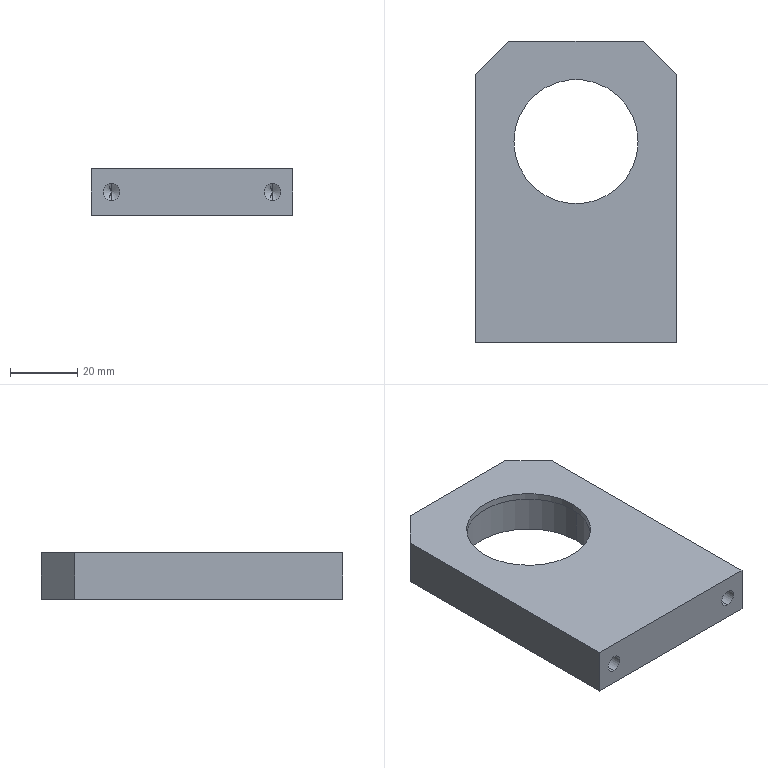Part | SolidWorks | features 3DProfileFeature 1, Chamfer 1, Extrusion 1, HoleWzd 1, ICE 1 | 1 solid | 21 faces | box 60 x 90 x 14 mm | volume 56400 mm3 | plane 9 | cylinder 8 | cone 4 | commonest cylinder face diameters 5 x4 37 x2 40 x2
STEP:
#1=CARTESIAN_POINT('',(-24.,-31.,2.5));
#2=VERTEX_POINT('',#1);
#3=CARTESIAN_POINT('',(-24.,-31.,-2.5));
#4=VERTEX_POINT('',#3);
#5=CARTESIAN_POINT('',(-24.,-31.,0.));
#6=DIRECTION('',(0.,-1.,0.));
#7=DIRECTION('',(0.,0.,-1.));
#8=AXIS2_PLACEMENT_3D('',#5,#6,#7);
#9=CIRCLE('',#8,2.5);
#10=EDGE_CURVE('',#2,#4,#9,.T.);
#11=ORIENTED_EDGE('',*,*,#10,.F.);
#12=CARTESIAN_POINT('',(-24.,-45.,2.5));
#13=VERTEX_POINT('',#12);
#14=CARTESIAN_POINT('',(-24.,-45.,2.5));
#15=DIRECTION('',(0.,-1.,0.));
#16=VECTOR('',#15,1000.);
#17=LINE('',#14,#16);
#18=EDGE_CURVE('',#2,#13,#17,.T.);
#19=ORIENTED_EDGE('',*,*,#18,.T.);
#20=CARTESIAN_POINT('',(-24.,-45.,-2.5));
#21=VERTEX_POINT('',#20);
#22=CARTESIAN_POINT('',(-24.,-45.,0.));
#23=DIRECTION('',(0.,-1.,0.));
#24=DIRECTION('',(0.,0.,-1.));
#25=AXIS2_PLACEMENT_3D('',#22,#23,#24);
#26=CIRCLE('',#25,2.5);
#27=EDGE_CURVE('',#13,#21,#26,.T.);
#28=ORIENTED_EDGE('',*,*,#27,.T.);
#29=CARTESIAN_POINT('',(-24.,-45.,-2.5));
#30=DIRECTION('',(0.,-1.,0.));
#31=VECTOR('',#30,1000.);
#32=LINE('',#29,#31);
#33=EDGE_CURVE('',#4,#21,#32,.T.);
#34=ORIENTED_EDGE('',*,*,#33,.F.);
#35=EDGE_LOOP('',(#11,#19,#28,#34));
#36=FACE_OUTER_BOUND('',#35,.T.);
#37=CARTESIAN_POINT('',(-24.,-45.,0.));
#38=DIRECTION('',(0.,-1.,0.));
#39=DIRECTION('',(0.,0.,-1.));
#40=AXIS2_PLACEMENT_3D('',#37,#38,#39);
#41=CYLINDRICAL_SURFACE('',#40,2.5);
#42=ADVANCED_FACE('',(#36),#41,.F.);
#43=CARTESIAN_POINT('',(-24.,-29.498,0.));
#44=VERTEX_POINT('',#43);
#45=CARTESIAN_POINT('',(-24.,-31.,-2.5));
#46=DIRECTION('',(0.,-0.515,-0.8572));
#47=VECTOR('',#46,1000.);
#48=LINE('',#45,#47);
#49=EDGE_CURVE('',#44,#4,#48,.T.);
#50=ORIENTED_EDGE('',*,*,#49,.F.);
#51=CARTESIAN_POINT('',(-24.,-31.,2.5));
#52=DIRECTION('',(0.,-0.515,0.8572));
#53=VECTOR('',#52,1000.);
#54=LINE('',#51,#53);
#55=EDGE_CURVE('',#44,#2,#54,.T.);
#56=ORIENTED_EDGE('',*,*,#55,.T.);
#57=ORIENTED_EDGE('',*,*,#10,.T.);
#58=EDGE_LOOP('',(#50,#56,#57));
#59=FACE_OUTER_BOUND('',#58,.T.);
#60=CARTESIAN_POINT('',(-24.,-31.,0.));
#61=DIRECTION('',(0.,-1.,0.));
#62=DIRECTION('',(0.,0.,-1.));
#63=AXIS2_PLACEMENT_3D('',#60,#61,#62);
#64=CONICAL_SURFACE('',#63,2.5,1.03);
#65=ADVANCED_FACE('',(#59),#64,.F.);
#66=CARTESIAN_POINT('',(24.,-31.,2.5));
#67=VERTEX_POINT('',#66);
#68=CARTESIAN_POINT('',(24.,-31.,-2.5));
#69=VERTEX_POINT('',#68);
#70=CARTESIAN_POINT('',(24.,-31.,0.));
#71=DIRECTION('',(0.,-1.,0.));
#72=DIRECTION('',(0.,0.,-1.));
#73=AXIS2_PLACEMENT_3D('',#70,#71,#72);
#74=CIRCLE('',#73,2.5);
#75=EDGE_CURVE('',#67,#69,#74,.T.);
#76=ORIENTED_EDGE('',*,*,#75,.F.);
#77=CARTESIAN_POINT('',(24.,-45.,2.5));
#78=VERTEX_POINT('',#77);
#79=CARTESIAN_POINT('',(24.,-45.,2.5));
#80=DIRECTION('',(0.,-1.,0.));
#81=VECTOR('',#80,1000.);
#82=LINE('',#79,#81);
#83=EDGE_CURVE('',#67,#78,#82,.T.);
#84=ORIENTED_EDGE('',*,*,#83,.T.);
#85=CARTESIAN_POINT('',(24.,-45.,-2.5));
#86=VERTEX_POINT('',#85);
#87=CARTESIAN_POINT('',(24.,-45.,0.));
#88=DIRECTION('',(0.,-1.,0.));
#89=DIRECTION('',(0.,0.,-1.));
#90=AXIS2_PLACEMENT_3D('',#87,#88,#89);
#91=CIRCLE('',#90,2.5);
#92=EDGE_CURVE('',#78,#86,#91,.T.);
#93=ORIENTED_EDGE('',*,*,#92,.T.);
#94=CARTESIAN_POINT('',(24.,-45.,-2.5));
#95=DIRECTION('',(0.,-1.,0.));
#96=VECTOR('',#95,1000.);
#97=LINE('',#94,#96);
#98=EDGE_CURVE('',#69,#86,#97,.T.);
#99=ORIENTED_EDGE('',*,*,#98,.F.);
#100=EDGE_LOOP('',(#76,#84,#93,#99));
#101=FACE_OUTER_BOUND('',#100,.T.);
#102=CARTESIAN_POINT('',(24.,-45.,0.));
#103=DIRECTION('',(0.,-1.,0.));
#104=DIRECTION('',(0.,0.,-1.));
#105=AXIS2_PLACEMENT_3D('',#102,#103,#104);
#106=CYLINDRICAL_SURFACE('',#105,2.5);
#107=ADVANCED_FACE('',(#101),#106,.F.);
#108=CARTESIAN_POINT('',(24.,-29.498,0.));
#109=VERTEX_POINT('',#108);
#110=CARTESIAN_POINT('',(24.,-31.,-2.5));
#111=DIRECTION('',(0.,-0.515,-0.8572));
#112=VECTOR('',#111,1000.);
#113=LINE('',#110,#112);
#114=EDGE_CURVE('',#109,#69,#113,.T.);
#115=ORIENTED_EDGE('',*,*,#114,.F.);
#116=CARTESIAN_POINT('',(24.,-31.,2.5));
#117=DIRECTION('',(0.,-0.515,0.8572));
#118=VECTOR('',#117,1000.);
#119=LINE('',#116,#118);
#120=EDGE_CURVE('',#109,#67,#119,.T.);
#121=ORIENTED_EDGE('',*,*,#120,.T.);
#122=ORIENTED_EDGE('',*,*,#75,.T.);
#123=EDGE_LOOP('',(#115,#121,#122));
#124=FACE_OUTER_BOUND('',#123,.T.);
#125=CARTESIAN_POINT('',(24.,-31.,0.));
#126=DIRECTION('',(0.,-1.,0.));
#127=DIRECTION('',(0.,0.,-1.));
#128=AXIS2_PLACEMENT_3D('',#125,#126,#127);
#129=CONICAL_SURFACE('',#128,2.5,1.03);
#130=ADVANCED_FACE('',(#124),#129,.F.);
#131=CARTESIAN_POINT('',(-18.5,15.,5.));
#132=VERTEX_POINT('',#131);
#133=CARTESIAN_POINT('',(18.5,15.,5.));
#134=VERTEX_POINT('',#133);
#135=CARTESIAN_POINT('',(0.,15.,5.));
#136=DIRECTION('',(0.,0.,1.));
#137=DIRECTION('',(1.,0.,0.));
#138=AXIS2_PLACEMENT_3D('',#135,#136,#137);
#139=CIRCLE('',#138,18.5);
#140=EDGE_CURVE('',#132,#134,#139,.T.);
#141=ORIENTED_EDGE('',*,*,#140,.F.);
#142=CARTESIAN_POINT('',(-18.5,15.,7.));
#143=VERTEX_POINT('',#142);
#144=CARTESIAN_POINT('',(-18.5,15.,5.));
#145=DIRECTION('',(0.,0.,1.));
#146=VECTOR('',#145,1000.);
#147=LINE('',#144,#146);
#148=EDGE_CURVE('',#132,#143,#147,.T.);
#149=ORIENTED_EDGE('',*,*,#148,.T.);
#150=CARTESIAN_POINT('',(18.5,15.,7.));
#151=VERTEX_POINT('',#150);
#152=CARTESIAN_POINT('',(0.,15.,7.));
#153=DIRECTION('',(0.,0.,1.));
#154=DIRECTION('',(1.,0.,0.));
#155=AXIS2_PLACEMENT_3D('',#152,#153,#154);
#156=CIRCLE('',#155,18.5);
#157=EDGE_CURVE('',#143,#151,#156,.T.);
#158=ORIENTED_EDGE('',*,*,#157,.T.);
#159=CARTESIAN_POINT('',(18.5,15.,5.));
#160=DIRECTION('',(0.,0.,1.));
#161=VECTOR('',#160,1000.);
#162=LINE('',#159,#161);
#163=EDGE_CURVE('',#134,#151,#162,.T.);
#164=ORIENTED_EDGE('',*,*,#163,.F.);
#165=EDGE_LOOP('',(#141,#149,#158,#164));
#166=FACE_OUTER_BOUND('',#165,.T.);
#167=CARTESIAN_POINT('',(0.,15.,5.));
#168=DIRECTION('',(0.,0.,1.));
#169=DIRECTION('',(1.,0.,0.));
#170=AXIS2_PLACEMENT_3D('',#167,#168,#169);
#171=CYLINDRICAL_SURFACE('',#170,18.5);
#172=ADVANCED_FACE('',(#166),#171,.F.);
#173=CARTESIAN_POINT('',(-20.,15.,5.));
#174=VERTEX_POINT('',#173);
#175=CARTESIAN_POINT('',(20.,15.,5.));
#176=VERTEX_POINT('',#175);
#177=CARTESIAN_POINT('',(0.,15.,5.));
#178=DIRECTION('',(0.,0.,1.));
#179=DIRECTION('',(1.,0.,0.));
#180=AXIS2_PLACEMENT_3D('',#177,#178,#179);
#181=CIRCLE('',#180,20.);
#182=EDGE_CURVE('',#174,#176,#181,.T.);
#183=ORIENTED_EDGE('',*,*,#182,.T.);
#184=CARTESIAN_POINT('',(20.,15.,-7.));
#185=VERTEX_POINT('',#184);
#186=CARTESIAN_POINT('',(20.,15.,7.));
#187=DIRECTION('',(0.,0.,-1.));
#188=VECTOR('',#187,1000.);
#189=LINE('',#186,#188);
#190=EDGE_CURVE('',#176,#185,#189,.T.);
#191=ORIENTED_EDGE('',*,*,#190,.T.);
#192=CARTESIAN_POINT('',(-20.,15.,-7.));
#193=VERTEX_POINT('',#192);
#194=CARTESIAN_POINT('',(0.,15.,-7.));
#195=DIRECTION('',(0.,0.,1.));
#196=DIRECTION('',(1.,0.,0.));
#197=AXIS2_PLACEMENT_3D('',#194,#195,#196);
#198=CIRCLE('',#197,20.);
#199=EDGE_CURVE('',#193,#185,#198,.T.);
#200=ORIENTED_EDGE('',*,*,#199,.F.);
#201=CARTESIAN_POINT('',(-20.,15.,7.));
#202=DIRECTION('',(0.,0.,-1.));
#203=VECTOR('',#202,1000.);
#204=LINE('',#201,#203);
#205=EDGE_CURVE('',#174,#193,#204,.T.);
#206=ORIENTED_EDGE('',*,*,#205,.F.);
#207=EDGE_LOOP('',(#183,#191,#200,#206));
#208=FACE_OUTER_BOUND('',#207,.T.);
#209=CARTESIAN_POINT('',(0.,15.,7.));
#210=DIRECTION('',(0.,0.,-1.));
#211=DIRECTION('',(-1.,0.,0.));
#212=AXIS2_PLACEMENT_3D('',#209,#210,#211);
#213=CYLINDRICAL_SURFACE('',#212,20.);
#214=ADVANCED_FACE('',(#208),#213,.F.);
#215=ORIENTED_EDGE('',*,*,#190,.F.);
#216=CARTESIAN_POINT('',(0.,15.,5.));
#217=DIRECTION('',(0.,0.,1.));
#218=DIRECTION('',(1.,0.,0.));
#219=AXIS2_PLACEMENT_3D('',#216,#217,#218);
#220=CIRCLE('',#219,20.);
#221=EDGE_CURVE('',#176,#174,#220,.T.);
#222=ORIENTED_EDGE('',*,*,#221,.T.);
#223=ORIENTED_EDGE('',*,*,#205,.T.);
#224=CARTESIAN_POINT('',(0.,15.,-7.));
#225=DIRECTION('',(0.,0.,1.));
#226=DIRECTION('',(1.,0.,0.));
#227=AXIS2_PLACEMENT_3D('',#224,#225,#226);
#228=CIRCLE('',#227,20.);
#229=EDGE_CURVE('',#185,#193,#228,.T.);
#230=ORIENTED_EDGE('',*,*,#229,.F.);
#231=EDGE_LOOP('',(#215,#222,#223,#230));
#232=FACE_OUTER_BOUND('',#231,.T.);
#233=CARTESIAN_POINT('',(0.,15.,7.));
#234=DIRECTION('',(0.,0.,-1.));
#235=DIRECTION('',(-1.,0.,0.));
#236=AXIS2_PLACEMENT_3D('',#233,#234,#235);
#237=CYLINDRICAL_SURFACE('',#236,20.);
#238=ADVANCED_FACE('',(#232),#237,.F.);
#239=CARTESIAN_POINT('',(30.,-45.,7.));
#240=VERTEX_POINT('',#239);
#241=CARTESIAN_POINT('',(30.,35.,7.));
#242=VERTEX_POINT('',#241);
#243=CARTESIAN_POINT('',(30.,-45.,7.));
#244=DIRECTION('',(0.,1.,0.));
#245=VECTOR('',#244,1000.);
#246=LINE('',#243,#245);
#247=EDGE_CURVE('',#240,#242,#246,.T.);
#248=ORIENTED_EDGE('',*,*,#247,.T.);
#249=CARTESIAN_POINT('',(20.,45.,7.));
#250=VERTEX_POINT('',#249);
#251=CARTESIAN_POINT('',(20.,45.,7.));
#252=DIRECTION('',(-0.7071,0.7071,0.));
#253=VECTOR('',#252,1000.);
#254=LINE('',#251,#253);
#255=EDGE_CURVE('',#242,#250,#254,.T.);
#256=ORIENTED_EDGE('',*,*,#255,.T.);
#257=CARTESIAN_POINT('',(-20.,45.,7.));
#258=VERTEX_POINT('',#257);
#259=CARTESIAN_POINT('',(-30.,45.,7.));
#260=DIRECTION('',(-1.,0.,0.));
#261=VECTOR('',#260,1000.);
#262=LINE('',#259,#261);
#263=EDGE_CURVE('',#250,#258,#262,.T.);
#264=ORIENTED_EDGE('',*,*,#263,.T.);
#265=CARTESIAN_POINT('',(-30.,35.,7.));
#266=VERTEX_POINT('',#265);
#267=CARTESIAN_POINT('',(-30.,35.,7.));
#268=DIRECTION('',(-0.7071,-0.7071,0.));
#269=VECTOR('',#268,1000.);
#270=LINE('',#267,#269);
#271=EDGE_CURVE('',#258,#266,#270,.T.);
#272=ORIENTED_EDGE('',*,*,#271,.T.);
#273=CARTESIAN_POINT('',(-30.,-45.,7.));
#274=VERTEX_POINT('',#273);
#275=CARTESIAN_POINT('',(-30.,-45.,7.));
#276=DIRECTION('',(0.,-1.,0.));
#277=VECTOR('',#276,1000.);
#278=LINE('',#275,#277);
#279=EDGE_CURVE('',#266,#274,#278,.T.);
#280=ORIENTED_EDGE('',*,*,#279,.T.);
#281=CARTESIAN_POINT('',(-30.,-45.,7.));
#282=DIRECTION('',(1.,0.,0.));
#283=VECTOR('',#282,1000.);
#284=LINE('',#281,#283);
#285=EDGE_CURVE('',#274,#240,#284,.T.);
#286=ORIENTED_EDGE('',*,*,#285,.T.);
#287=EDGE_LOOP('',(#248,#256,#264,#272,#280,#286));
#288=FACE_OUTER_BOUND('',#287,.T.);
#289=CARTESIAN_POINT('',(0.,15.,7.));
#290=DIRECTION('',(0.,0.,1.));
#291=DIRECTION('',(1.,0.,0.));
#292=AXIS2_PLACEMENT_3D('',#289,#290,#291);
#293=CIRCLE('',#292,18.5);
#294=EDGE_CURVE('',#151,#143,#293,.T.);
#295=ORIENTED_EDGE('',*,*,#294,.F.);
#296=ORIENTED_EDGE('',*,*,#157,.F.);
#297=EDGE_LOOP('',(#295,#296));
#298=FACE_BOUND('',#297,.T.);
#299=CARTESIAN_POINT('',(0.,0.,7.));
#300=DIRECTION('',(0.,0.,-1.));
#301=DIRECTION('',(-1.,0.,0.));
#302=AXIS2_PLACEMENT_3D('',#299,#300,#301);
#303=PLANE('',#302);
#304=ADVANCED_FACE('',(#288,#298),#303,.F.);
#305=CARTESIAN_POINT('',(20.,45.,-7.));
#306=VERTEX_POINT('',#305);
#307=CARTESIAN_POINT('',(-20.,45.,-7.));
#308=VERTEX_POINT('',#307);
#309=CARTESIAN_POINT('',(-30.,45.,-7.));
#310=DIRECTION('',(-1.,0.,0.));
#311=VECTOR('',#310,1000.);
#312=LINE('',#309,#311);
#313=EDGE_CURVE('',#306,#308,#312,.T.);
#314=ORIENTED_EDGE('',*,*,#313,.F.);
#315=CARTESIAN_POINT('',(30.,35.,-7.));
#316=VERTEX_POINT('',#315);
#317=CARTESIAN_POINT('',(32.5,32.5,-7.));
#318=DIRECTION('',(0.7071,-0.7071,0.));
#319=VECTOR('',#318,1000.);
#320=LINE('',#317,#319);
#321=EDGE_CURVE('',#306,#316,#320,.T.);
#322=ORIENTED_EDGE('',*,*,#321,.T.);
#323=CARTESIAN_POINT('',(30.,-45.,-7.));
#324=VERTEX_POINT('',#323);
#325=CARTESIAN_POINT('',(30.,-45.,-7.));
#326=DIRECTION('',(0.,1.,0.));
#327=VECTOR('',#326,1000.);
#328=LINE('',#325,#327);
#329=EDGE_CURVE('',#324,#316,#328,.T.);
#330=ORIENTED_EDGE('',*,*,#329,.F.);
#331=CARTESIAN_POINT('',(-30.,-45.,-7.));
#332=VERTEX_POINT('',#331);
#333=CARTESIAN_POINT('',(-30.,-45.,-7.));
#334=DIRECTION('',(1.,0.,0.));
#335=VECTOR('',#334,1000.);
#336=LINE('',#333,#335);
#337=EDGE_CURVE('',#332,#324,#336,.T.);
#338=ORIENTED_EDGE('',*,*,#337,.F.);
#339=CARTESIAN_POINT('',(-30.,35.,-7.));
#340=VERTEX_POINT('',#339);
#341=CARTESIAN_POINT('',(-30.,-45.,-7.));
#342=DIRECTION('',(0.,-1.,0.));
#343=VECTOR('',#342,1000.);
#344=LINE('',#341,#343);
#345=EDGE_CURVE('',#340,#332,#344,.T.);
#346=ORIENTED_EDGE('',*,*,#345,.F.);
#347=CARTESIAN_POINT('',(-32.5,32.5,-7.));
#348=DIRECTION('',(0.7071,0.7071,0.));
#349=VECTOR('',#348,1000.);
#350=LINE('',#347,#349);
#351=EDGE_CURVE('',#340,#308,#350,.T.);
#352=ORIENTED_EDGE('',*,*,#351,.T.);
#353=EDGE_LOOP('',(#314,#322,#330,#338,#346,#352));
#354=FACE_OUTER_BOUND('',#353,.T.);
#355=ORIENTED_EDGE('',*,*,#199,.T.);
#356=ORIENTED_EDGE('',*,*,#229,.T.);
#357=EDGE_LOOP('',(#355,#356));
#358=FACE_BOUND('',#357,.T.);
#359=CARTESIAN_POINT('',(0.,0.,-7.));
#360=DIRECTION('',(0.,0.,-1.));
#361=DIRECTION('',(-1.,0.,0.));
#362=AXIS2_PLACEMENT_3D('',#359,#360,#361);
#363=PLANE('',#362);
#364=ADVANCED_FACE('',(#354,#358),#363,.T.);
#365=ORIENTED_EDGE('',*,*,#329,.T.);
#366=CARTESIAN_POINT('',(30.,35.,7.));
#367=DIRECTION('',(0.,0.,1.));
#368=VECTOR('',#367,1000.);
#369=LINE('',#366,#368);
#370=EDGE_CURVE('',#316,#242,#369,.T.);
#371=ORIENTED_EDGE('',*,*,#370,.T.);
#372=ORIENTED_EDGE('',*,*,#247,.F.);
#373=CARTESIAN_POINT('',(30.,-45.,7.));
#374=DIRECTION('',(0.,0.,-1.));
#375=VECTOR('',#374,1000.);
#376=LINE('',#373,#375);
#377=EDGE_CURVE('',#240,#324,#376,.T.);
#378=ORIENTED_EDGE('',*,*,#377,.T.);
#379=EDGE_LOOP('',(#365,#371,#372,#378));
#380=FACE_OUTER_BOUND('',#379,.T.);
#381=CARTESIAN_POINT('',(30.,-45.,7.));
#382=DIRECTION('',(-1.,0.,0.));
#383=DIRECTION('',(0.,0.,1.));
#384=AXIS2_PLACEMENT_3D('',#381,#382,#383);
#385=PLANE('',#384);
#386=ADVANCED_FACE('',(#380),#385,.F.);
#387=ORIENTED_EDGE('',*,*,#263,.F.);
#388=CARTESIAN_POINT('',(20.,45.,7.));
#389=DIRECTION('',(0.,0.,-1.));
#390=VECTOR('',#389,1000.);
#391=LINE('',#388,#390);
#392=EDGE_CURVE('',#250,#306,#391,.T.);
#393=ORIENTED_EDGE('',*,*,#392,.T.);
#394=ORIENTED_EDGE('',*,*,#313,.T.);
#395=CARTESIAN_POINT('',(-20.,45.,7.));
#396=DIRECTION('',(0.,0.,1.));
#397=VECTOR('',#396,1000.);
#398=LINE('',#395,#397);
#399=EDGE_CURVE('',#308,#258,#398,.T.);
#400=ORIENTED_EDGE('',*,*,#399,.T.);
#401=EDGE_LOOP('',(#387,#393,#394,#400));
#402=FACE_OUTER_BOUND('',#401,.T.);
#403=CARTESIAN_POINT('',(-30.,45.,7.));
#404=DIRECTION('',(0.,-1.,0.));
#405=DIRECTION('',(1.,0.,0.));
#406=AXIS2_PLACEMENT_3D('',#403,#404,#405);
#407=PLANE('',#406);
#408=ADVANCED_FACE('',(#402),#407,.F.);
#409=ORIENTED_EDGE('',*,*,#279,.F.);
#410=CARTESIAN_POINT('',(-30.,35.,7.));
#411=DIRECTION('',(0.,0.,-1.));
#412=VECTOR('',#411,1000.);
#413=LINE('',#410,#412);
#414=EDGE_CURVE('',#266,#340,#413,.T.);
#415=ORIENTED_EDGE('',*,*,#414,.T.);
#416=ORIENTED_EDGE('',*,*,#345,.T.);
#417=CARTESIAN_POINT('',(-30.,-45.,7.));
#418=DIRECTION('',(0.,0.,-1.));
#419=VECTOR('',#418,1000.);
#420=LINE('',#417,#419);
#421=EDGE_CURVE('',#274,#332,#420,.T.);
#422=ORIENTED_EDGE('',*,*,#421,.F.);
#423=EDGE_LOOP('',(#409,#415,#416,#422));
#424=FACE_OUTER_BOUND('',#423,.T.);
#425=CARTESIAN_POINT('',(-30.,-45.,7.));
#426=DIRECTION('',(1.,0.,0.));
#427=DIRECTION('',(0.,0.,-1.));
#428=AXIS2_PLACEMENT_3D('',#425,#426,#427);
#429=PLANE('',#428);
#430=ADVANCED_FACE('',(#424),#429,.F.);
#431=CARTESIAN_POINT('',(-24.,-45.,0.));
#432=DIRECTION('',(0.,-1.,0.));
#433=DIRECTION('',(0.,0.,-1.));
#434=AXIS2_PLACEMENT_3D('',#431,#432,#433);
#435=CIRCLE('',#434,2.5);
#436=EDGE_CURVE('',#21,#13,#435,.T.);
#437=ORIENTED_EDGE('',*,*,#436,.F.);
#438=ORIENTED_EDGE('',*,*,#27,.F.);
#439=EDGE_LOOP('',(#437,#438));
#440=FACE_BOUND('',#439,.T.);
#441=CARTESIAN_POINT('',(24.,-45.,0.));
#442=DIRECTION('',(0.,-1.,0.));
#443=DIRECTION('',(0.,0.,-1.));
#444=AXIS2_PLACEMENT_3D('',#441,#442,#443);
#445=CIRCLE('',#444,2.5);
#446=EDGE_CURVE('',#86,#78,#445,.T.);
#447=ORIENTED_EDGE('',*,*,#446,.F.);
#448=ORIENTED_EDGE('',*,*,#92,.F.);
#449=EDGE_LOOP('',(#447,#448));
#450=FACE_BOUND('',#449,.T.);
#451=ORIENTED_EDGE('',*,*,#337,.T.);
#452=ORIENTED_EDGE('',*,*,#377,.F.);
#453=ORIENTED_EDGE('',*,*,#285,.F.);
#454=ORIENTED_EDGE('',*,*,#421,.T.);
#455=EDGE_LOOP('',(#451,#452,#453,#454));
#456=FACE_OUTER_BOUND('',#455,.T.);
#457=CARTESIAN_POINT('',(-30.,-45.,7.));
#458=DIRECTION('',(0.,1.,0.));
#459=DIRECTION('',(0.,0.,1.));
#460=AXIS2_PLACEMENT_3D('',#457,#458,#459);
#461=PLANE('',#460);
#462=ADVANCED_FACE('',(#440,#450,#456),#461,.F.);
#463=CARTESIAN_POINT('',(0.,15.,5.));
#464=DIRECTION('',(0.,0.,1.));
#465=DIRECTION('',(1.,0.,0.));
#466=AXIS2_PLACEMENT_3D('',#463,#464,#465);
#467=CIRCLE('',#466,18.5);
#468=EDGE_CURVE('',#134,#132,#467,.T.);
#469=ORIENTED_EDGE('',*,*,#468,.T.);
#470=ORIENTED_EDGE('',*,*,#140,.T.);
#471=EDGE_LOOP('',(#469,#470));
#472=FACE_BOUND('',#471,.T.);
#473=ORIENTED_EDGE('',*,*,#182,.F.);
#474=ORIENTED_EDGE('',*,*,#221,.F.);
#475=EDGE_LOOP('',(#473,#474));
#476=FACE_OUTER_BOUND('',#475,.T.);
#477=CARTESIAN_POINT('',(0.,15.,5.));
#478=DIRECTION('',(0.,0.,1.));
#479=DIRECTION('',(1.,0.,0.));
#480=AXIS2_PLACEMENT_3D('',#477,#478,#479);
#481=PLANE('',#480);
#482=ADVANCED_FACE('',(#472,#476),#481,.F.);
#483=ORIENTED_EDGE('',*,*,#148,.F.);
#484=ORIENTED_EDGE('',*,*,#468,.F.);
#485=ORIENTED_EDGE('',*,*,#163,.T.);
#486=ORIENTED_EDGE('',*,*,#294,.T.);
#487=EDGE_LOOP('',(#483,#484,#485,#486));
#488=FACE_OUTER_BOUND('',#487,.T.);
#489=CARTESIAN_POINT('',(0.,15.,5.));
#490=DIRECTION('',(0.,0.,1.));
#491=DIRECTION('',(1.,0.,0.));
#492=AXIS2_PLACEMENT_3D('',#489,#490,#491);
#493=CYLINDRICAL_SURFACE('',#492,18.5);
#494=ADVANCED_FACE('',(#488),#493,.F.);
#495=ORIENTED_EDGE('',*,*,#255,.F.);
#496=ORIENTED_EDGE('',*,*,#370,.F.);
#497=ORIENTED_EDGE('',*,*,#321,.F.);
#498=ORIENTED_EDGE('',*,*,#392,.F.);
#499=EDGE_LOOP('',(#495,#496,#497,#498));
#500=FACE_OUTER_BOUND('',#499,.T.);
#501=CARTESIAN_POINT('',(20.,45.,7.));
#502=DIRECTION('',(-0.7071,-0.7071,0.));
#503=DIRECTION('',(0.,0.,-1.));
#504=AXIS2_PLACEMENT_3D('',#501,#502,#503);
#505=PLANE('',#504);
#506=ADVANCED_FACE('',(#500),#505,.F.);
#507=ORIENTED_EDGE('',*,*,#271,.F.);
#508=ORIENTED_EDGE('',*,*,#399,.F.);
#509=ORIENTED_EDGE('',*,*,#351,.F.);
#510=ORIENTED_EDGE('',*,*,#414,.F.);
#511=EDGE_LOOP('',(#507,#508,#509,#510));
#512=FACE_OUTER_BOUND('',#511,.T.);
#513=CARTESIAN_POINT('',(-30.,35.,7.));
#514=DIRECTION('',(0.7071,-0.7071,0.));
#515=DIRECTION('',(0.,0.,-1.));
#516=AXIS2_PLACEMENT_3D('',#513,#514,#515);
#517=PLANE('',#516);
#518=ADVANCED_FACE('',(#512),#517,.F.);
#519=ORIENTED_EDGE('',*,*,#120,.F.);
#520=ORIENTED_EDGE('',*,*,#114,.T.);
#521=CARTESIAN_POINT('',(24.,-31.,0.));
#522=DIRECTION('',(0.,-1.,0.));
#523=DIRECTION('',(0.,0.,-1.));
#524=AXIS2_PLACEMENT_3D('',#521,#522,#523);
#525=CIRCLE('',#524,2.5);
#526=EDGE_CURVE('',#69,#67,#525,.T.);
#527=ORIENTED_EDGE('',*,*,#526,.T.);
#528=EDGE_LOOP('',(#519,#520,#527));
#529=FACE_OUTER_BOUND('',#528,.T.);
#530=CARTESIAN_POINT('',(24.,-31.,0.));
#531=DIRECTION('',(0.,-1.,0.));
#532=DIRECTION('',(0.,0.,-1.));
#533=AXIS2_PLACEMENT_3D('',#530,#531,#532);
#534=CONICAL_SURFACE('',#533,2.5,1.03);
#535=ADVANCED_FACE('',(#529),#534,.F.);
#536=ORIENTED_EDGE('',*,*,#83,.F.);
#537=ORIENTED_EDGE('',*,*,#526,.F.);
#538=ORIENTED_EDGE('',*,*,#98,.T.);
#539=ORIENTED_EDGE('',*,*,#446,.T.);
#540=EDGE_LOOP('',(#536,#537,#538,#539));
#541=FACE_OUTER_BOUND('',#540,.T.);
#542=CARTESIAN_POINT('',(24.,-45.,0.));
#543=DIRECTION('',(0.,-1.,0.));
#544=DIRECTION('',(0.,0.,-1.));
#545=AXIS2_PLACEMENT_3D('',#542,#543,#544);
#546=CYLINDRICAL_SURFACE('',#545,2.5);
#547=ADVANCED_FACE('',(#541),#546,.F.);
#548=ORIENTED_EDGE('',*,*,#55,.F.);
#549=ORIENTED_EDGE('',*,*,#49,.T.);
#550=CARTESIAN_POINT('',(-24.,-31.,0.));
#551=DIRECTION('',(0.,-1.,0.));
#552=DIRECTION('',(0.,0.,-1.));
#553=AXIS2_PLACEMENT_3D('',#550,#551,#552);
#554=CIRCLE('',#553,2.5);
#555=EDGE_CURVE('',#4,#2,#554,.T.);
#556=ORIENTED_EDGE('',*,*,#555,.T.);
#557=EDGE_LOOP('',(#548,#549,#556));
#558=FACE_OUTER_BOUND('',#557,.T.);
#559=CARTESIAN_POINT('',(-24.,-31.,0.));
#560=DIRECTION('',(0.,-1.,0.));
#561=DIRECTION('',(0.,0.,-1.));
#562=AXIS2_PLACEMENT_3D('',#559,#560,#561);
#563=CONICAL_SURFACE('',#562,2.5,1.03);
#564=ADVANCED_FACE('',(#558),#563,.F.);
#565=ORIENTED_EDGE('',*,*,#18,.F.);
#566=ORIENTED_EDGE('',*,*,#555,.F.);
#567=ORIENTED_EDGE('',*,*,#33,.T.);
#568=ORIENTED_EDGE('',*,*,#436,.T.);
#569=EDGE_LOOP('',(#565,#566,#567,#568));
#570=FACE_OUTER_BOUND('',#569,.T.);
#571=CARTESIAN_POINT('',(-24.,-45.,0.));
#572=DIRECTION('',(0.,-1.,0.));
#573=DIRECTION('',(0.,0.,-1.));
#574=AXIS2_PLACEMENT_3D('',#571,#572,#573);
#575=CYLINDRICAL_SURFACE('',#574,2.5);
#576=ADVANCED_FACE('',(#570),#575,.F.);
#577=CLOSED_SHELL('',(#42,#65,#107,#130,#172,#214,#238,#304,#364,#386,#408,#430,#462,#482,#494,#506,#518,#535,#547,#564,#576));
#578=MANIFOLD_SOLID_BREP('',#577);
#579=CARTESIAN_POINT('',(0.,0.,0.));
#580=DIRECTION('',(0.,0.,1.));
#581=DIRECTION('',(1.,0.,0.));
#582=AXIS2_PLACEMENT_3D('',#579,#580,#581);
#583=(LENGTH_UNIT()NAMED_UNIT(*)SI_UNIT(.MILLI.,.METRE.));
#584=UNCERTAINTY_MEASURE_WITH_UNIT(LENGTH_MEASURE(0.00001),#583,'','');
#585=(NAMED_UNIT(*)PLANE_ANGLE_UNIT()SI_UNIT($,.RADIAN.));
#586=(NAMED_UNIT(*)SI_UNIT($,.STERADIAN.)SOLID_ANGLE_UNIT());
#587=(GEOMETRIC_REPRESENTATION_CONTEXT(3)GLOBAL_UNCERTAINTY_ASSIGNED_CONTEXT((#584))GLOBAL_UNIT_ASSIGNED_CONTEXT((#583,#585,#586))REPRESENTATION_CONTEXT('',''));
#588=ADVANCED_BREP_SHAPE_REPRESENTATION('',(#578,#582),#587);